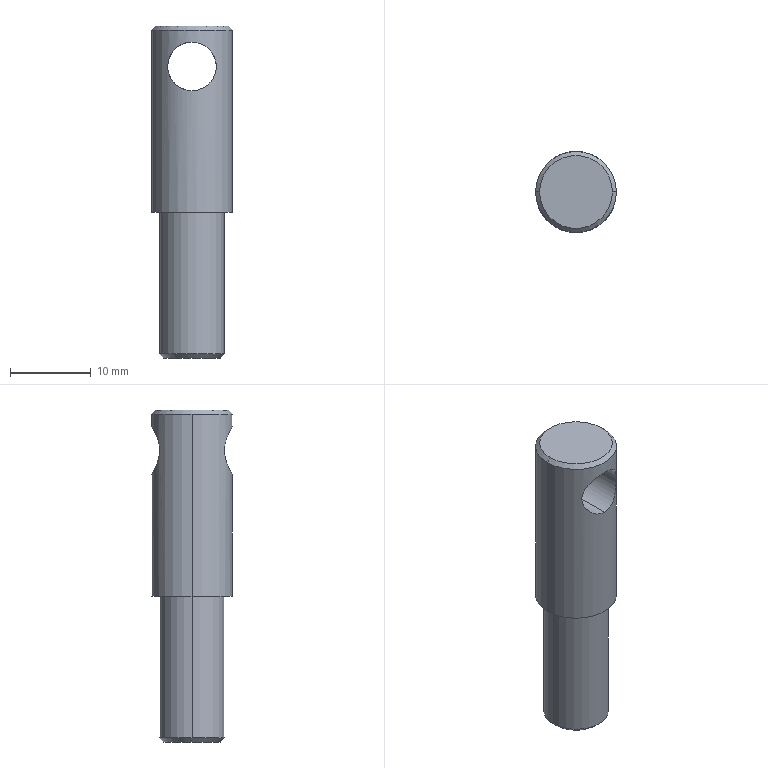Part | SolidWorks | features ICE 2, Chamfer 1, Extrusion 1 | 1 solid | 13 faces | box 10 x 10 x 41 mm | volume 2435 mm3 | cylinder 6 | cone 4 | plane 3 | commonest cylinder face diameters 6 x2 8 x2 10 x2
STEP:
#1=CARTESIAN_POINT('',(0.,-5.,15.));
#2=VERTEX_POINT('',#1);
#3=CARTESIAN_POINT('',(0.,-5.,21.));
#4=VERTEX_POINT('',#3);
#5=CARTESIAN_POINT('',(0.,-5.,15.));
#6=CARTESIAN_POINT('',(-0.2026,-5.,15.));
#7=CARTESIAN_POINT('',(-0.4018,-4.988,15.02));
#8=CARTESIAN_POINT('',(-0.7938,-4.941,15.1));
#9=CARTESIAN_POINT('',(-0.9867,-4.905,15.16));
#10=CARTESIAN_POINT('',(-1.348,-4.818,15.313));
#11=CARTESIAN_POINT('',(-1.521,-4.766,15.407));
#12=CARTESIAN_POINT('',(-1.843,-4.651,15.625));
#13=CARTESIAN_POINT('',(-1.99,-4.589,15.747));
#14=CARTESIAN_POINT('',(-2.26,-4.463,16.018));
#15=CARTESIAN_POINT('',(-2.383,-4.397,16.167));
#16=CARTESIAN_POINT('',(-2.596,-4.275,16.485));
#17=CARTESIAN_POINT('',(-2.688,-4.217,16.653));
#18=CARTESIAN_POINT('',(-2.84,-4.116,17.014));
#19=CARTESIAN_POINT('',(-2.899,-4.074,17.204));
#20=CARTESIAN_POINT('',(-2.979,-4.016,17.594));
#21=CARTESIAN_POINT('',(-3.,-4.,17.798));
#22=CARTESIAN_POINT('',(-3.,-4.,18.201));
#23=CARTESIAN_POINT('',(-2.98,-4.015,18.4));
#24=CARTESIAN_POINT('',(-2.9,-4.073,18.794));
#25=CARTESIAN_POINT('',(-2.841,-4.115,18.983));
#26=CARTESIAN_POINT('',(-2.689,-4.216,19.344));
#27=CARTESIAN_POINT('',(-2.596,-4.275,19.516));
#28=CARTESIAN_POINT('',(-2.382,-4.398,19.834));
#29=CARTESIAN_POINT('',(-2.26,-4.462,19.982));
#30=CARTESIAN_POINT('',(-1.988,-4.59,20.255));
#31=CARTESIAN_POINT('',(-1.84,-4.652,20.377));
#32=CARTESIAN_POINT('',(-1.522,-4.766,20.592));
#33=CARTESIAN_POINT('',(-1.349,-4.818,20.687));
#34=CARTESIAN_POINT('',(-0.9853,-4.906,20.84));
#35=CARTESIAN_POINT('',(-0.797,-4.94,20.899));
#36=CARTESIAN_POINT('',(-0.4074,-4.987,20.979));
#37=CARTESIAN_POINT('',(-0.2033,-5.,21.));
#38=CARTESIAN_POINT('',(0.,-5.,21.));
#39=B_SPLINE_CURVE_WITH_KNOTS('',3,(#5,#6,#7,#8,#9,#10,#11,#12,#13,#14,#15,#16,#17,#18,#19,#20,#21,#22,#23,#24,#25,#26,#27,#28,#29,#30,#31,#32,#33,#34,#35,#36,#37,#38),.UNSPECIFIED.,.F.,.F.,(4,2,2,2,2,2,2,2,2,2,2,2,2,2,2,2,4),(0.009625,0.01023,0.01083,0.01143,0.01203,0.01263,0.01323,0.01383,0.01443,0.01503,0.01563,0.01623,0.01683,0.01743,0.01803,0.01863,0.01923),.UNSPECIFIED.);
#40=EDGE_CURVE('',#2,#4,#39,.T.);
#41=ORIENTED_EDGE('',*,*,#40,.F.);
#42=CARTESIAN_POINT('',(0.,5.,15.));
#43=VERTEX_POINT('',#42);
#44=CARTESIAN_POINT('',(0.,-5.,15.));
#45=DIRECTION('',(0.,1.,0.));
#46=VECTOR('',#45,1000.);
#47=LINE('',#44,#46);
#48=EDGE_CURVE('',#2,#43,#47,.T.);
#49=ORIENTED_EDGE('',*,*,#48,.T.);
#50=CARTESIAN_POINT('',(0.,5.,21.));
#51=VERTEX_POINT('',#50);
#52=CARTESIAN_POINT('',(0.,5.,21.));
#53=CARTESIAN_POINT('',(-0.2037,5.,21.));
#54=CARTESIAN_POINT('',(-0.4031,4.988,20.979));
#55=CARTESIAN_POINT('',(-0.794,4.94,20.9));
#56=CARTESIAN_POINT('',(-0.9871,4.905,20.84));
#57=CARTESIAN_POINT('',(-1.53,4.775,20.61));
#58=CARTESIAN_POINT('',(-1.856,4.652,20.388));
#59=CARTESIAN_POINT('',(-2.26,4.463,19.982));
#60=CARTESIAN_POINT('',(-2.383,4.397,19.833));
#61=CARTESIAN_POINT('',(-2.597,4.275,19.514));
#62=CARTESIAN_POINT('',(-2.688,4.217,19.346));
#63=CARTESIAN_POINT('',(-2.839,4.117,18.988));
#64=CARTESIAN_POINT('',(-2.899,4.074,18.796));
#65=CARTESIAN_POINT('',(-2.979,4.016,18.405));
#66=CARTESIAN_POINT('',(-3.,4.,18.204));
#67=CARTESIAN_POINT('',(-3.,4.,17.798));
#68=CARTESIAN_POINT('',(-2.98,4.015,17.598));
#69=CARTESIAN_POINT('',(-2.9,4.073,17.207));
#70=CARTESIAN_POINT('',(-2.841,4.116,17.015));
#71=CARTESIAN_POINT('',(-2.689,4.216,16.656));
#72=CARTESIAN_POINT('',(-2.596,4.275,16.484));
#73=CARTESIAN_POINT('',(-2.381,4.399,16.164));
#74=CARTESIAN_POINT('',(-2.259,4.463,16.017));
#75=CARTESIAN_POINT('',(-1.988,4.59,15.745));
#76=CARTESIAN_POINT('',(-1.839,4.653,15.622));
#77=CARTESIAN_POINT('',(-1.52,4.766,15.406));
#78=CARTESIAN_POINT('',(-1.35,4.818,15.314));
#79=CARTESIAN_POINT('',(-0.8028,4.949,15.082));
#80=CARTESIAN_POINT('',(-0.406,5.,15.));
#81=CARTESIAN_POINT('',(0.,5.,15.));
#82=B_SPLINE_CURVE_WITH_KNOTS('',3,(#52,#53,#54,#55,#56,#57,#58,#59,#60,#61,#62,#63,#64,#65,#66,#67,#68,#69,#70,#71,#72,#73,#74,#75,#76,#77,#78,#79,#80,#81),.UNSPECIFIED.,.F.,.F.,(4,2,2,2,2,2,2,2,2,2,2,2,2,2,4),(0.,0.0006015,0.001203,0.002406,0.003008,0.003609,0.004211,0.004812,0.005414,0.006015,0.006617,0.007219,0.00782,0.008422,0.009625),.UNSPECIFIED.);
#83=EDGE_CURVE('',#51,#43,#82,.T.);
#84=ORIENTED_EDGE('',*,*,#83,.F.);
#85=CARTESIAN_POINT('',(0.,-5.,21.));
#86=DIRECTION('',(0.,1.,0.));
#87=VECTOR('',#86,1000.);
#88=LINE('',#85,#87);
#89=EDGE_CURVE('',#4,#51,#88,.T.);
#90=ORIENTED_EDGE('',*,*,#89,.F.);
#91=EDGE_LOOP('',(#41,#49,#84,#90));
#92=FACE_OUTER_BOUND('',#91,.T.);
#93=CARTESIAN_POINT('',(0.,-5.,18.));
#94=DIRECTION('',(0.,1.,0.));
#95=DIRECTION('',(0.,0.,1.));
#96=AXIS2_PLACEMENT_3D('',#93,#94,#95);
#97=CYLINDRICAL_SURFACE('',#96,3.);
#98=ADVANCED_FACE('',(#92),#97,.F.);
#99=CARTESIAN_POINT('',(-3.5,0.,-18.));
#100=VERTEX_POINT('',#99);
#101=CARTESIAN_POINT('',(3.5,0.,-18.));
#102=VERTEX_POINT('',#101);
#103=CARTESIAN_POINT('',(0.,0.,-18.));
#104=DIRECTION('',(0.,0.,-1.));
#105=DIRECTION('',(-1.,0.,0.));
#106=AXIS2_PLACEMENT_3D('',#103,#104,#105);
#107=CIRCLE('',#106,3.5);
#108=EDGE_CURVE('',#100,#102,#107,.T.);
#109=ORIENTED_EDGE('',*,*,#108,.F.);
#110=CARTESIAN_POINT('',(-4.,0.,-17.5));
#111=VERTEX_POINT('',#110);
#112=CARTESIAN_POINT('',(-3.5,0.,-18.));
#113=DIRECTION('',(-0.7071,0.,0.7071));
#114=VECTOR('',#113,1000.);
#115=LINE('',#112,#114);
#116=EDGE_CURVE('',#100,#111,#115,.T.);
#117=ORIENTED_EDGE('',*,*,#116,.T.);
#118=CARTESIAN_POINT('',(4.,0.,-17.5));
#119=VERTEX_POINT('',#118);
#120=CARTESIAN_POINT('',(0.,0.,-17.5));
#121=DIRECTION('',(0.,0.,1.));
#122=DIRECTION('',(-1.,0.,0.));
#123=AXIS2_PLACEMENT_3D('',#120,#121,#122);
#124=CIRCLE('',#123,4.);
#125=EDGE_CURVE('',#119,#111,#124,.T.);
#126=ORIENTED_EDGE('',*,*,#125,.F.);
#127=CARTESIAN_POINT('',(3.5,0.,-18.));
#128=DIRECTION('',(0.7071,0.,0.7071));
#129=VECTOR('',#128,1000.);
#130=LINE('',#127,#129);
#131=EDGE_CURVE('',#102,#119,#130,.T.);
#132=ORIENTED_EDGE('',*,*,#131,.F.);
#133=EDGE_LOOP('',(#109,#117,#126,#132));
#134=FACE_OUTER_BOUND('',#133,.T.);
#135=CARTESIAN_POINT('',(0.,0.,-18.));
#136=DIRECTION('',(0.,0.,1.));
#137=DIRECTION('',(1.,0.,0.));
#138=AXIS2_PLACEMENT_3D('',#135,#136,#137);
#139=CONICAL_SURFACE('',#138,3.5,0.7854);
#140=ADVANCED_FACE('',(#134),#139,.T.);
#141=CARTESIAN_POINT('',(4.5,0.,23.));
#142=VERTEX_POINT('',#141);
#143=CARTESIAN_POINT('',(-4.5,0.,23.));
#144=VERTEX_POINT('',#143);
#145=CARTESIAN_POINT('',(0.,0.,23.));
#146=DIRECTION('',(0.,0.,1.));
#147=DIRECTION('',(1.,0.,0.));
#148=AXIS2_PLACEMENT_3D('',#145,#146,#147);
#149=CIRCLE('',#148,4.5);
#150=EDGE_CURVE('',#142,#144,#149,.T.);
#151=ORIENTED_EDGE('',*,*,#150,.F.);
#152=CARTESIAN_POINT('',(5.,0.,22.5));
#153=VERTEX_POINT('',#152);
#154=CARTESIAN_POINT('',(4.5,0.,23.));
#155=DIRECTION('',(0.7071,0.,-0.7071));
#156=VECTOR('',#155,1000.);
#157=LINE('',#154,#156);
#158=EDGE_CURVE('',#142,#153,#157,.T.);
#159=ORIENTED_EDGE('',*,*,#158,.T.);
#160=CARTESIAN_POINT('',(-5.,0.,22.5));
#161=VERTEX_POINT('',#160);
#162=CARTESIAN_POINT('',(0.,0.,22.5));
#163=DIRECTION('',(0.,0.,-1.));
#164=DIRECTION('',(1.,0.,0.));
#165=AXIS2_PLACEMENT_3D('',#162,#163,#164);
#166=CIRCLE('',#165,5.);
#167=EDGE_CURVE('',#161,#153,#166,.T.);
#168=ORIENTED_EDGE('',*,*,#167,.F.);
#169=CARTESIAN_POINT('',(-4.5,0.,23.));
#170=DIRECTION('',(-0.7071,0.,-0.7071));
#171=VECTOR('',#170,1000.);
#172=LINE('',#169,#171);
#173=EDGE_CURVE('',#144,#161,#172,.T.);
#174=ORIENTED_EDGE('',*,*,#173,.F.);
#175=EDGE_LOOP('',(#151,#159,#168,#174));
#176=FACE_OUTER_BOUND('',#175,.T.);
#177=CARTESIAN_POINT('',(0.,0.,23.));
#178=DIRECTION('',(0.,0.,-1.));
#179=DIRECTION('',(-1.,0.,0.));
#180=AXIS2_PLACEMENT_3D('',#177,#178,#179);
#181=CONICAL_SURFACE('',#180,4.5,0.7854);
#182=ADVANCED_FACE('',(#176),#181,.T.);
#183=ORIENTED_EDGE('',*,*,#125,.T.);
#184=CARTESIAN_POINT('',(-4.,0.,0.));
#185=VERTEX_POINT('',#184);
#186=CARTESIAN_POINT('',(-4.,0.,-18.));
#187=DIRECTION('',(0.,0.,1.));
#188=VECTOR('',#187,1000.);
#189=LINE('',#186,#188);
#190=EDGE_CURVE('',#111,#185,#189,.T.);
#191=ORIENTED_EDGE('',*,*,#190,.T.);
#192=CARTESIAN_POINT('',(4.,0.,0.));
#193=VERTEX_POINT('',#192);
#194=CARTESIAN_POINT('',(0.,0.,0.));
#195=DIRECTION('',(0.,0.,-1.));
#196=DIRECTION('',(-1.,0.,0.));
#197=AXIS2_PLACEMENT_3D('',#194,#195,#196);
#198=CIRCLE('',#197,4.);
#199=EDGE_CURVE('',#185,#193,#198,.T.);
#200=ORIENTED_EDGE('',*,*,#199,.T.);
#201=CARTESIAN_POINT('',(4.,0.,-18.));
#202=DIRECTION('',(0.,0.,1.));
#203=VECTOR('',#202,1000.);
#204=LINE('',#201,#203);
#205=EDGE_CURVE('',#119,#193,#204,.T.);
#206=ORIENTED_EDGE('',*,*,#205,.F.);
#207=EDGE_LOOP('',(#183,#191,#200,#206));
#208=FACE_OUTER_BOUND('',#207,.T.);
#209=CARTESIAN_POINT('',(0.,0.,-18.));
#210=DIRECTION('',(0.,0.,1.));
#211=DIRECTION('',(1.,0.,0.));
#212=AXIS2_PLACEMENT_3D('',#209,#210,#211);
#213=CYLINDRICAL_SURFACE('',#212,4.);
#214=ADVANCED_FACE('',(#208),#213,.T.);
#215=ORIENTED_EDGE('',*,*,#83,.T.);
#216=CARTESIAN_POINT('',(0.,5.,15.));
#217=CARTESIAN_POINT('',(0.2026,5.,15.));
#218=CARTESIAN_POINT('',(0.4018,4.988,15.02));
#219=CARTESIAN_POINT('',(0.7938,4.941,15.1));
#220=CARTESIAN_POINT('',(0.9867,4.905,15.16));
#221=CARTESIAN_POINT('',(1.348,4.818,15.313));
#222=CARTESIAN_POINT('',(1.521,4.766,15.407));
#223=CARTESIAN_POINT('',(1.843,4.651,15.625));
#224=CARTESIAN_POINT('',(1.99,4.589,15.747));
#225=CARTESIAN_POINT('',(2.26,4.463,16.018));
#226=CARTESIAN_POINT('',(2.383,4.397,16.167));
#227=CARTESIAN_POINT('',(2.596,4.275,16.485));
#228=CARTESIAN_POINT('',(2.688,4.217,16.653));
#229=CARTESIAN_POINT('',(2.84,4.116,17.014));
#230=CARTESIAN_POINT('',(2.899,4.074,17.204));
#231=CARTESIAN_POINT('',(2.979,4.016,17.594));
#232=CARTESIAN_POINT('',(3.,4.,17.798));
#233=CARTESIAN_POINT('',(3.,4.,18.201));
#234=CARTESIAN_POINT('',(2.98,4.015,18.4));
#235=CARTESIAN_POINT('',(2.9,4.073,18.794));
#236=CARTESIAN_POINT('',(2.841,4.115,18.983));
#237=CARTESIAN_POINT('',(2.689,4.216,19.344));
#238=CARTESIAN_POINT('',(2.596,4.275,19.516));
#239=CARTESIAN_POINT('',(2.382,4.398,19.834));
#240=CARTESIAN_POINT('',(2.26,4.462,19.982));
#241=CARTESIAN_POINT('',(1.988,4.59,20.255));
#242=CARTESIAN_POINT('',(1.84,4.652,20.377));
#243=CARTESIAN_POINT('',(1.522,4.766,20.592));
#244=CARTESIAN_POINT('',(1.349,4.818,20.687));
#245=CARTESIAN_POINT('',(0.9853,4.906,20.84));
#246=CARTESIAN_POINT('',(0.797,4.94,20.899));
#247=CARTESIAN_POINT('',(0.4074,4.987,20.979));
#248=CARTESIAN_POINT('',(0.2033,5.,21.));
#249=CARTESIAN_POINT('',(0.,5.,21.));
#250=B_SPLINE_CURVE_WITH_KNOTS('',3,(#216,#217,#218,#219,#220,#221,#222,#223,#224,#225,#226,#227,#228,#229,#230,#231,#232,#233,#234,#235,#236,#237,#238,#239,#240,#241,#242,#243,#244,#245,#246,#247,#248,#249),.UNSPECIFIED.,.F.,.F.,(4,2,2,2,2,2,2,2,2,2,2,2,2,2,2,2,4),(0.009625,0.01023,0.01083,0.01143,0.01203,0.01263,0.01323,0.01383,0.01443,0.01503,0.01563,0.01623,0.01683,0.01743,0.01803,0.01863,0.01923),.UNSPECIFIED.);
#251=EDGE_CURVE('',#43,#51,#250,.T.);
#252=ORIENTED_EDGE('',*,*,#251,.T.);
#253=EDGE_LOOP('',(#215,#252));
#254=FACE_BOUND('',#253,.T.);
#255=ORIENTED_EDGE('',*,*,#167,.T.);
#256=CARTESIAN_POINT('',(5.,0.,0.));
#257=VERTEX_POINT('',#256);
#258=CARTESIAN_POINT('',(5.,0.,23.));
#259=DIRECTION('',(0.,0.,-1.));
#260=VECTOR('',#259,1000.);
#261=LINE('',#258,#260);
#262=EDGE_CURVE('',#153,#257,#261,.T.);
#263=ORIENTED_EDGE('',*,*,#262,.T.);
#264=CARTESIAN_POINT('',(-5.,0.,0.));
#265=VERTEX_POINT('',#264);
#266=CARTESIAN_POINT('',(0.,0.,0.));
#267=DIRECTION('',(0.,0.,1.));
#268=DIRECTION('',(1.,0.,0.));
#269=AXIS2_PLACEMENT_3D('',#266,#267,#268);
#270=CIRCLE('',#269,5.);
#271=EDGE_CURVE('',#257,#265,#270,.T.);
#272=ORIENTED_EDGE('',*,*,#271,.T.);
#273=CARTESIAN_POINT('',(-5.,0.,23.));
#274=DIRECTION('',(0.,0.,-1.));
#275=VECTOR('',#274,1000.);
#276=LINE('',#273,#275);
#277=EDGE_CURVE('',#161,#265,#276,.T.);
#278=ORIENTED_EDGE('',*,*,#277,.F.);
#279=EDGE_LOOP('',(#255,#263,#272,#278));
#280=FACE_OUTER_BOUND('',#279,.T.);
#281=CARTESIAN_POINT('',(0.,0.,23.));
#282=DIRECTION('',(0.,0.,-1.));
#283=DIRECTION('',(-1.,0.,0.));
#284=AXIS2_PLACEMENT_3D('',#281,#282,#283);
#285=CYLINDRICAL_SURFACE('',#284,5.);
#286=ADVANCED_FACE('',(#254,#280),#285,.T.);
#287=ORIENTED_EDGE('',*,*,#262,.F.);
#288=CARTESIAN_POINT('',(0.,0.,22.5));
#289=DIRECTION('',(0.,0.,-1.));
#290=DIRECTION('',(1.,0.,0.));
#291=AXIS2_PLACEMENT_3D('',#288,#289,#290);
#292=CIRCLE('',#291,5.);
#293=EDGE_CURVE('',#153,#161,#292,.T.);
#294=ORIENTED_EDGE('',*,*,#293,.T.);
#295=ORIENTED_EDGE('',*,*,#277,.T.);
#296=CARTESIAN_POINT('',(0.,0.,0.));
#297=DIRECTION('',(0.,0.,1.));
#298=DIRECTION('',(1.,0.,0.));
#299=AXIS2_PLACEMENT_3D('',#296,#297,#298);
#300=CIRCLE('',#299,5.);
#301=EDGE_CURVE('',#265,#257,#300,.T.);
#302=ORIENTED_EDGE('',*,*,#301,.T.);
#303=EDGE_LOOP('',(#287,#294,#295,#302));
#304=FACE_OUTER_BOUND('',#303,.T.);
#305=CARTESIAN_POINT('',(0.,-5.,21.));
#306=CARTESIAN_POINT('',(0.2037,-5.,21.));
#307=CARTESIAN_POINT('',(0.4031,-4.988,20.979));
#308=CARTESIAN_POINT('',(0.794,-4.94,20.9));
#309=CARTESIAN_POINT('',(0.9871,-4.905,20.84));
#310=CARTESIAN_POINT('',(1.53,-4.775,20.61));
#311=CARTESIAN_POINT('',(1.856,-4.652,20.388));
#312=CARTESIAN_POINT('',(2.26,-4.463,19.982));
#313=CARTESIAN_POINT('',(2.383,-4.397,19.833));
#314=CARTESIAN_POINT('',(2.597,-4.275,19.514));
#315=CARTESIAN_POINT('',(2.688,-4.217,19.346));
#316=CARTESIAN_POINT('',(2.839,-4.117,18.988));
#317=CARTESIAN_POINT('',(2.899,-4.074,18.796));
#318=CARTESIAN_POINT('',(2.979,-4.016,18.405));
#319=CARTESIAN_POINT('',(3.,-4.,18.204));
#320=CARTESIAN_POINT('',(3.,-4.,17.798));
#321=CARTESIAN_POINT('',(2.98,-4.015,17.598));
#322=CARTESIAN_POINT('',(2.9,-4.073,17.207));
#323=CARTESIAN_POINT('',(2.841,-4.116,17.015));
#324=CARTESIAN_POINT('',(2.689,-4.216,16.656));
#325=CARTESIAN_POINT('',(2.596,-4.275,16.484));
#326=CARTESIAN_POINT('',(2.381,-4.399,16.164));
#327=CARTESIAN_POINT('',(2.259,-4.463,16.017));
#328=CARTESIAN_POINT('',(1.988,-4.59,15.745));
#329=CARTESIAN_POINT('',(1.839,-4.653,15.622));
#330=CARTESIAN_POINT('',(1.52,-4.766,15.406));
#331=CARTESIAN_POINT('',(1.35,-4.818,15.314));
#332=CARTESIAN_POINT('',(0.8028,-4.949,15.082));
#333=CARTESIAN_POINT('',(0.406,-5.,15.));
#334=CARTESIAN_POINT('',(0.,-5.,15.));
#335=B_SPLINE_CURVE_WITH_KNOTS('',3,(#305,#306,#307,#308,#309,#310,#311,#312,#313,#314,#315,#316,#317,#318,#319,#320,#321,#322,#323,#324,#325,#326,#327,#328,#329,#330,#331,#332,#333,#334),.UNSPECIFIED.,.F.,.F.,(4,2,2,2,2,2,2,2,2,2,2,2,2,2,4),(0.,0.0006015,0.001203,0.002406,0.003008,0.003609,0.004211,0.004812,0.005414,0.006015,0.006617,0.007219,0.00782,0.008422,0.009625),.UNSPECIFIED.);
#336=EDGE_CURVE('',#4,#2,#335,.T.);
#337=ORIENTED_EDGE('',*,*,#336,.T.);
#338=ORIENTED_EDGE('',*,*,#40,.T.);
#339=EDGE_LOOP('',(#337,#338));
#340=FACE_BOUND('',#339,.T.);
#341=CARTESIAN_POINT('',(0.,0.,23.));
#342=DIRECTION('',(0.,0.,-1.));
#343=DIRECTION('',(-1.,0.,0.));
#344=AXIS2_PLACEMENT_3D('',#341,#342,#343);
#345=CYLINDRICAL_SURFACE('',#344,5.);
#346=ADVANCED_FACE('',(#304,#340),#345,.T.);
#347=CARTESIAN_POINT('',(0.,0.,23.));
#348=DIRECTION('',(0.,0.,1.));
#349=DIRECTION('',(1.,0.,0.));
#350=AXIS2_PLACEMENT_3D('',#347,#348,#349);
#351=CIRCLE('',#350,4.5);
#352=EDGE_CURVE('',#144,#142,#351,.T.);
#353=ORIENTED_EDGE('',*,*,#352,.T.);
#354=ORIENTED_EDGE('',*,*,#150,.T.);
#355=EDGE_LOOP('',(#353,#354));
#356=FACE_OUTER_BOUND('',#355,.T.);
#357=CARTESIAN_POINT('',(0.,0.,23.));
#358=DIRECTION('',(0.,0.,1.));
#359=DIRECTION('',(1.,0.,0.));
#360=AXIS2_PLACEMENT_3D('',#357,#358,#359);
#361=PLANE('',#360);
#362=ADVANCED_FACE('',(#356),#361,.T.);
#363=CARTESIAN_POINT('',(0.,0.,0.));
#364=DIRECTION('',(0.,0.,-1.));
#365=DIRECTION('',(-1.,0.,0.));
#366=AXIS2_PLACEMENT_3D('',#363,#364,#365);
#367=CIRCLE('',#366,4.);
#368=EDGE_CURVE('',#193,#185,#367,.T.);
#369=ORIENTED_EDGE('',*,*,#368,.F.);
#370=ORIENTED_EDGE('',*,*,#199,.F.);
#371=EDGE_LOOP('',(#369,#370));
#372=FACE_BOUND('',#371,.T.);
#373=ORIENTED_EDGE('',*,*,#301,.F.);
#374=ORIENTED_EDGE('',*,*,#271,.F.);
#375=EDGE_LOOP('',(#373,#374));
#376=FACE_OUTER_BOUND('',#375,.T.);
#377=CARTESIAN_POINT('',(0.,0.,0.));
#378=DIRECTION('',(0.,0.,1.));
#379=DIRECTION('',(1.,0.,0.));
#380=AXIS2_PLACEMENT_3D('',#377,#378,#379);
#381=PLANE('',#380);
#382=ADVANCED_FACE('',(#372,#376),#381,.F.);
#383=ORIENTED_EDGE('',*,*,#190,.F.);
#384=CARTESIAN_POINT('',(0.,0.,-17.5));
#385=DIRECTION('',(0.,0.,1.));
#386=DIRECTION('',(-1.,0.,0.));
#387=AXIS2_PLACEMENT_3D('',#384,#385,#386);
#388=CIRCLE('',#387,4.);
#389=EDGE_CURVE('',#111,#119,#388,.T.);
#390=ORIENTED_EDGE('',*,*,#389,.T.);
#391=ORIENTED_EDGE('',*,*,#205,.T.);
#392=ORIENTED_EDGE('',*,*,#368,.T.);
#393=EDGE_LOOP('',(#383,#390,#391,#392));
#394=FACE_OUTER_BOUND('',#393,.T.);
#395=CARTESIAN_POINT('',(0.,0.,-18.));
#396=DIRECTION('',(0.,0.,1.));
#397=DIRECTION('',(1.,0.,0.));
#398=AXIS2_PLACEMENT_3D('',#395,#396,#397);
#399=CYLINDRICAL_SURFACE('',#398,4.);
#400=ADVANCED_FACE('',(#394),#399,.T.);
#401=CARTESIAN_POINT('',(0.,0.,-18.));
#402=DIRECTION('',(0.,0.,-1.));
#403=DIRECTION('',(-1.,0.,0.));
#404=AXIS2_PLACEMENT_3D('',#401,#402,#403);
#405=CIRCLE('',#404,3.5);
#406=EDGE_CURVE('',#102,#100,#405,.T.);
#407=ORIENTED_EDGE('',*,*,#406,.T.);
#408=ORIENTED_EDGE('',*,*,#108,.T.);
#409=EDGE_LOOP('',(#407,#408));
#410=FACE_OUTER_BOUND('',#409,.T.);
#411=CARTESIAN_POINT('',(0.,0.,-18.));
#412=DIRECTION('',(0.,0.,-1.));
#413=DIRECTION('',(-1.,0.,0.));
#414=AXIS2_PLACEMENT_3D('',#411,#412,#413);
#415=PLANE('',#414);
#416=ADVANCED_FACE('',(#410),#415,.T.);
#417=ORIENTED_EDGE('',*,*,#158,.F.);
#418=ORIENTED_EDGE('',*,*,#352,.F.);
#419=ORIENTED_EDGE('',*,*,#173,.T.);
#420=ORIENTED_EDGE('',*,*,#293,.F.);
#421=EDGE_LOOP('',(#417,#418,#419,#420));
#422=FACE_OUTER_BOUND('',#421,.T.);
#423=CARTESIAN_POINT('',(0.,0.,23.));
#424=DIRECTION('',(0.,0.,-1.));
#425=DIRECTION('',(-1.,0.,0.));
#426=AXIS2_PLACEMENT_3D('',#423,#424,#425);
#427=CONICAL_SURFACE('',#426,4.5,0.7854);
#428=ADVANCED_FACE('',(#422),#427,.T.);
#429=ORIENTED_EDGE('',*,*,#116,.F.);
#430=ORIENTED_EDGE('',*,*,#406,.F.);
#431=ORIENTED_EDGE('',*,*,#131,.T.);
#432=ORIENTED_EDGE('',*,*,#389,.F.);
#433=EDGE_LOOP('',(#429,#430,#431,#432));
#434=FACE_OUTER_BOUND('',#433,.T.);
#435=CARTESIAN_POINT('',(0.,0.,-18.));
#436=DIRECTION('',(0.,0.,1.));
#437=DIRECTION('',(1.,0.,0.));
#438=AXIS2_PLACEMENT_3D('',#435,#436,#437);
#439=CONICAL_SURFACE('',#438,3.5,0.7854);
#440=ADVANCED_FACE('',(#434),#439,.T.);
#441=ORIENTED_EDGE('',*,*,#48,.F.);
#442=ORIENTED_EDGE('',*,*,#336,.F.);
#443=ORIENTED_EDGE('',*,*,#89,.T.);
#444=ORIENTED_EDGE('',*,*,#251,.F.);
#445=EDGE_LOOP('',(#441,#442,#443,#444));
#446=FACE_OUTER_BOUND('',#445,.T.);
#447=CARTESIAN_POINT('',(0.,-5.,18.));
#448=DIRECTION('',(0.,1.,0.));
#449=DIRECTION('',(0.,0.,1.));
#450=AXIS2_PLACEMENT_3D('',#447,#448,#449);
#451=CYLINDRICAL_SURFACE('',#450,3.);
#452=ADVANCED_FACE('',(#446),#451,.F.);
#453=CLOSED_SHELL('',(#98,#140,#182,#214,#286,#346,#362,#382,#400,#416,#428,#440,#452));
#454=MANIFOLD_SOLID_BREP('',#453);
#455=CARTESIAN_POINT('',(0.,0.,0.));
#456=DIRECTION('',(0.,0.,1.));
#457=DIRECTION('',(1.,0.,0.));
#458=AXIS2_PLACEMENT_3D('',#455,#456,#457);
#459=(LENGTH_UNIT()NAMED_UNIT(*)SI_UNIT(.MILLI.,.METRE.));
#460=UNCERTAINTY_MEASURE_WITH_UNIT(LENGTH_MEASURE(0.00001),#459,'','');
#461=(NAMED_UNIT(*)PLANE_ANGLE_UNIT()SI_UNIT($,.RADIAN.));
#462=(NAMED_UNIT(*)SI_UNIT($,.STERADIAN.)SOLID_ANGLE_UNIT());
#463=(GEOMETRIC_REPRESENTATION_CONTEXT(3)GLOBAL_UNCERTAINTY_ASSIGNED_CONTEXT((#460))GLOBAL_UNIT_ASSIGNED_CONTEXT((#459,#461,#462))REPRESENTATION_CONTEXT('',''));
#464=ADVANCED_BREP_SHAPE_REPRESENTATION('',(#454,#458),#463);